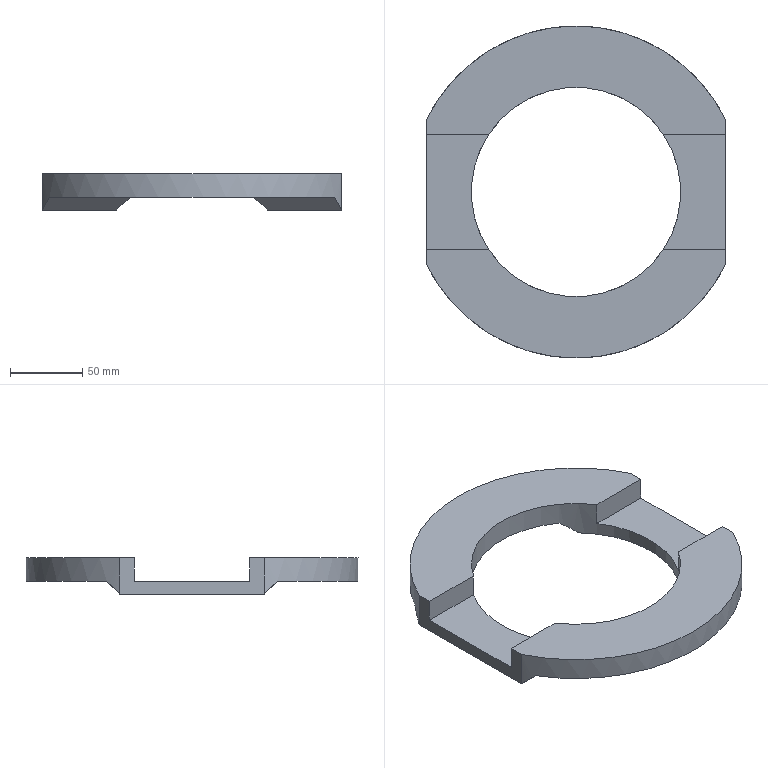Part | NX | features 掩护梁 2 | 1 solid | 21 faces | box 207.123 x 230 x 25 mm | volume 362169 mm3 | plane 18 | cylinder 3 | commonest cylinder face diameters 230 x2 145 x1
STEP:
#1=CARTESIAN_POINT('',(-1870.619,3715.447,-663.771));
#2=VERTEX_POINT('',#1);
#3=CARTESIAN_POINT('',(-1870.619,3715.447,-688.771));
#4=VERTEX_POINT('',#3);
#5=CARTESIAN_POINT('',(-1870.619,3715.447,-688.771));
#6=DIRECTION('',(0.,0.,1.));
#7=VECTOR('',#6,1000.);
#8=LINE('',#5,#7);
#9=EDGE_CURVE('',#2,#4,#8,.F.);
#10=ORIENTED_EDGE('',*,*,#9,.F.);
#11=CARTESIAN_POINT('',(-2077.742,3715.447,-663.771));
#12=VERTEX_POINT('',#11);
#13=CARTESIAN_POINT('',(-1974.181,3765.447,-663.771));
#14=DIRECTION('',(0.,0.,1.));
#15=DIRECTION('',(1.,0.,0.));
#16=AXIS2_PLACEMENT_3D('',#13,#14,#15);
#17=CIRCLE('',#16,115.);
#18=EDGE_CURVE('',#12,#2,#17,.T.);
#19=ORIENTED_EDGE('',*,*,#18,.F.);
#20=CARTESIAN_POINT('',(-2077.742,3715.447,-688.771));
#21=VERTEX_POINT('',#20);
#22=CARTESIAN_POINT('',(-2077.742,3715.447,-688.771));
#23=DIRECTION('',(0.,0.,1.));
#24=VECTOR('',#23,1000.);
#25=LINE('',#22,#24);
#26=EDGE_CURVE('',#21,#12,#25,.T.);
#27=ORIENTED_EDGE('',*,*,#26,.F.);
#28=CARTESIAN_POINT('',(-2072.893,3706.447,-679.771));
#29=VERTEX_POINT('',#28);
#30=CARTESIAN_POINT('',(-1974.181,3765.447,-738.771));
#31=DIRECTION('',(0.,-0.7071,-0.7071));
#32=DIRECTION('',(0.,-0.7071,0.7071));
#33=AXIS2_PLACEMENT_3D('',#30,#31,#32);
#34=ELLIPSE('',#33,162.635,115.);
#35=EDGE_CURVE('',#21,#29,#34,.F.);
#36=ORIENTED_EDGE('',*,*,#35,.T.);
#37=CARTESIAN_POINT('',(-1875.469,3706.447,-679.771));
#38=VERTEX_POINT('',#37);
#39=CARTESIAN_POINT('',(-1974.181,3765.447,-679.771));
#40=DIRECTION('',(0.,0.,-1.));
#41=DIRECTION('',(-1.,0.,0.));
#42=AXIS2_PLACEMENT_3D('',#39,#40,#41);
#43=CIRCLE('',#42,115.);
#44=EDGE_CURVE('',#29,#38,#43,.F.);
#45=ORIENTED_EDGE('',*,*,#44,.T.);
#46=CARTESIAN_POINT('',(-1974.181,3765.447,-738.771));
#47=DIRECTION('',(0.,-0.7071,-0.7071));
#48=DIRECTION('',(0.,-0.7071,0.7071));
#49=AXIS2_PLACEMENT_3D('',#46,#47,#48);
#50=ELLIPSE('',#49,162.635,115.);
#51=EDGE_CURVE('',#38,#4,#50,.F.);
#52=ORIENTED_EDGE('',*,*,#51,.T.);
#53=EDGE_LOOP('',(#10,#19,#27,#36,#45,#52));
#54=FACE_BOUND('',#53,.T.);
#55=CARTESIAN_POINT('',(-1974.181,3765.447,-688.771));
#56=DIRECTION('',(0.,0.,1.));
#57=DIRECTION('',(1.,0.,0.));
#58=AXIS2_PLACEMENT_3D('',#55,#56,#57);
#59=CYLINDRICAL_SURFACE('',#58,115.);
#60=ADVANCED_FACE('',(#54),#59,.T.);
#61=CARTESIAN_POINT('',(-1870.619,3815.447,-688.771));
#62=VERTEX_POINT('',#61);
#63=CARTESIAN_POINT('',(-1870.619,3815.447,-663.771));
#64=VERTEX_POINT('',#63);
#65=CARTESIAN_POINT('',(-1870.619,3815.447,-688.771));
#66=DIRECTION('',(0.,0.,1.));
#67=VECTOR('',#66,1000.);
#68=LINE('',#65,#67);
#69=EDGE_CURVE('',#62,#64,#68,.T.);
#70=ORIENTED_EDGE('',*,*,#69,.F.);
#71=CARTESIAN_POINT('',(-1875.469,3824.447,-679.771));
#72=VERTEX_POINT('',#71);
#73=CARTESIAN_POINT('',(-1974.181,3765.447,-738.771));
#74=DIRECTION('',(0.,0.7071,-0.7071));
#75=DIRECTION('',(0.,0.7071,0.7071));
#76=AXIS2_PLACEMENT_3D('',#73,#74,#75);
#77=ELLIPSE('',#76,162.635,115.);
#78=EDGE_CURVE('',#62,#72,#77,.F.);
#79=ORIENTED_EDGE('',*,*,#78,.T.);
#80=CARTESIAN_POINT('',(-2072.893,3824.447,-679.771));
#81=VERTEX_POINT('',#80);
#82=CARTESIAN_POINT('',(-1974.181,3765.447,-679.771));
#83=DIRECTION('',(0.,0.,-1.));
#84=DIRECTION('',(-1.,0.,0.));
#85=AXIS2_PLACEMENT_3D('',#82,#83,#84);
#86=CIRCLE('',#85,115.);
#87=EDGE_CURVE('',#72,#81,#86,.F.);
#88=ORIENTED_EDGE('',*,*,#87,.T.);
#89=CARTESIAN_POINT('',(-2077.742,3815.447,-688.771));
#90=VERTEX_POINT('',#89);
#91=CARTESIAN_POINT('',(-1974.181,3765.447,-738.771));
#92=DIRECTION('',(0.,0.7071,-0.7071));
#93=DIRECTION('',(0.,0.7071,0.7071));
#94=AXIS2_PLACEMENT_3D('',#91,#92,#93);
#95=ELLIPSE('',#94,162.635,115.);
#96=EDGE_CURVE('',#81,#90,#95,.F.);
#97=ORIENTED_EDGE('',*,*,#96,.T.);
#98=CARTESIAN_POINT('',(-2077.742,3815.447,-663.771));
#99=VERTEX_POINT('',#98);
#100=CARTESIAN_POINT('',(-2077.742,3815.447,-688.771));
#101=DIRECTION('',(0.,0.,1.));
#102=VECTOR('',#101,1000.);
#103=LINE('',#100,#102);
#104=EDGE_CURVE('',#99,#90,#103,.F.);
#105=ORIENTED_EDGE('',*,*,#104,.F.);
#106=CARTESIAN_POINT('',(-1974.181,3765.447,-663.771));
#107=DIRECTION('',(0.,0.,1.));
#108=DIRECTION('',(1.,0.,0.));
#109=AXIS2_PLACEMENT_3D('',#106,#107,#108);
#110=CIRCLE('',#109,115.);
#111=EDGE_CURVE('',#64,#99,#110,.T.);
#112=ORIENTED_EDGE('',*,*,#111,.F.);
#113=EDGE_LOOP('',(#70,#79,#88,#97,#105,#112));
#114=FACE_BOUND('',#113,.T.);
#115=CARTESIAN_POINT('',(-1974.181,3765.447,-688.771));
#116=DIRECTION('',(0.,0.,1.));
#117=DIRECTION('',(1.,0.,0.));
#118=AXIS2_PLACEMENT_3D('',#115,#116,#117);
#119=CYLINDRICAL_SURFACE('',#118,115.);
#120=ADVANCED_FACE('',(#114),#119,.T.);
#121=CARTESIAN_POINT('',(-2026.681,3715.447,-688.771));
#122=VERTEX_POINT('',#121);
#123=CARTESIAN_POINT('',(-2140.181,3715.447,-688.771));
#124=DIRECTION('',(1.,0.,0.));
#125=VECTOR('',#124,1000.);
#126=LINE('',#123,#125);
#127=EDGE_CURVE('',#21,#122,#126,.T.);
#128=ORIENTED_EDGE('',*,*,#127,.F.);
#129=CARTESIAN_POINT('',(-2077.742,3884.447,-688.771));
#130=DIRECTION('',(0.,-1.,0.));
#131=VECTOR('',#130,1000.);
#132=LINE('',#129,#131);
#133=EDGE_CURVE('',#90,#21,#132,.T.);
#134=ORIENTED_EDGE('',*,*,#133,.F.);
#135=CARTESIAN_POINT('',(-2026.681,3815.447,-688.771));
#136=VERTEX_POINT('',#135);
#137=CARTESIAN_POINT('',(-2140.181,3815.447,-688.771));
#138=DIRECTION('',(1.,0.,0.));
#139=VECTOR('',#138,1000.);
#140=LINE('',#137,#139);
#141=EDGE_CURVE('',#90,#136,#140,.T.);
#142=ORIENTED_EDGE('',*,*,#141,.T.);
#143=CARTESIAN_POINT('',(-1974.181,3765.447,-688.771));
#144=DIRECTION('',(0.,0.,1.));
#145=DIRECTION('',(1.,0.,0.));
#146=AXIS2_PLACEMENT_3D('',#143,#144,#145);
#147=CIRCLE('',#146,72.5);
#148=EDGE_CURVE('',#136,#122,#147,.T.);
#149=ORIENTED_EDGE('',*,*,#148,.T.);
#150=EDGE_LOOP('',(#128,#134,#142,#149));
#151=FACE_BOUND('',#150,.T.);
#152=CARTESIAN_POINT('',(-1974.181,3765.447,-688.771));
#153=DIRECTION('',(0.,0.,1.));
#154=DIRECTION('',(1.,0.,0.));
#155=AXIS2_PLACEMENT_3D('',#152,#153,#154);
#156=PLANE('',#155);
#157=ADVANCED_FACE('',(#151),#156,.F.);
#158=CARTESIAN_POINT('',(-1921.681,3815.447,-688.771));
#159=VERTEX_POINT('',#158);
#160=CARTESIAN_POINT('',(-2140.181,3815.447,-688.771));
#161=DIRECTION('',(1.,0.,0.));
#162=VECTOR('',#161,1000.);
#163=LINE('',#160,#162);
#164=EDGE_CURVE('',#159,#62,#163,.T.);
#165=ORIENTED_EDGE('',*,*,#164,.T.);
#166=CARTESIAN_POINT('',(-1870.619,3884.447,-688.771));
#167=DIRECTION('',(0.,-1.,0.));
#168=VECTOR('',#167,1000.);
#169=LINE('',#166,#168);
#170=EDGE_CURVE('',#62,#4,#169,.T.);
#171=ORIENTED_EDGE('',*,*,#170,.T.);
#172=CARTESIAN_POINT('',(-1921.681,3715.447,-688.771));
#173=VERTEX_POINT('',#172);
#174=CARTESIAN_POINT('',(-2140.181,3715.447,-688.771));
#175=DIRECTION('',(1.,0.,0.));
#176=VECTOR('',#175,1000.);
#177=LINE('',#174,#176);
#178=EDGE_CURVE('',#173,#4,#177,.T.);
#179=ORIENTED_EDGE('',*,*,#178,.F.);
#180=CARTESIAN_POINT('',(-1974.181,3765.447,-688.771));
#181=DIRECTION('',(0.,0.,1.));
#182=DIRECTION('',(1.,0.,0.));
#183=AXIS2_PLACEMENT_3D('',#180,#181,#182);
#184=CIRCLE('',#183,72.5);
#185=EDGE_CURVE('',#173,#159,#184,.T.);
#186=ORIENTED_EDGE('',*,*,#185,.T.);
#187=EDGE_LOOP('',(#165,#171,#179,#186));
#188=FACE_BOUND('',#187,.T.);
#189=CARTESIAN_POINT('',(-1974.181,3765.447,-688.771));
#190=DIRECTION('',(0.,0.,1.));
#191=DIRECTION('',(1.,0.,0.));
#192=AXIS2_PLACEMENT_3D('',#189,#190,#191);
#193=PLANE('',#192);
#194=ADVANCED_FACE('',(#188),#193,.F.);
#195=CARTESIAN_POINT('',(-1870.619,3725.447,-663.771));
#196=VERTEX_POINT('',#195);
#197=CARTESIAN_POINT('',(-1870.619,3884.447,-663.771));
#198=DIRECTION('',(0.,-1.,0.));
#199=VECTOR('',#198,1000.);
#200=LINE('',#197,#199);
#201=EDGE_CURVE('',#196,#2,#200,.T.);
#202=ORIENTED_EDGE('',*,*,#201,.F.);
#203=CARTESIAN_POINT('',(-1913.714,3725.447,-663.771));
#204=VERTEX_POINT('',#203);
#205=CARTESIAN_POINT('',(-2140.181,3725.447,-663.771));
#206=DIRECTION('',(1.,0.,0.));
#207=VECTOR('',#206,1000.);
#208=LINE('',#205,#207);
#209=EDGE_CURVE('',#204,#196,#208,.T.);
#210=ORIENTED_EDGE('',*,*,#209,.F.);
#211=CARTESIAN_POINT('',(-2034.648,3725.447,-663.771));
#212=VERTEX_POINT('',#211);
#213=CARTESIAN_POINT('',(-1974.181,3765.447,-663.771));
#214=DIRECTION('',(0.,0.,1.));
#215=DIRECTION('',(1.,0.,0.));
#216=AXIS2_PLACEMENT_3D('',#213,#214,#215);
#217=CIRCLE('',#216,72.5);
#218=EDGE_CURVE('',#212,#204,#217,.T.);
#219=ORIENTED_EDGE('',*,*,#218,.F.);
#220=CARTESIAN_POINT('',(-2077.742,3725.447,-663.771));
#221=VERTEX_POINT('',#220);
#222=CARTESIAN_POINT('',(-2140.181,3725.447,-663.771));
#223=DIRECTION('',(1.,0.,0.));
#224=VECTOR('',#223,1000.);
#225=LINE('',#222,#224);
#226=EDGE_CURVE('',#221,#212,#225,.T.);
#227=ORIENTED_EDGE('',*,*,#226,.F.);
#228=CARTESIAN_POINT('',(-2077.742,3884.447,-663.771));
#229=DIRECTION('',(0.,-1.,0.));
#230=VECTOR('',#229,1000.);
#231=LINE('',#228,#230);
#232=EDGE_CURVE('',#221,#12,#231,.T.);
#233=ORIENTED_EDGE('',*,*,#232,.T.);
#234=ORIENTED_EDGE('',*,*,#18,.T.);
#235=EDGE_LOOP('',(#202,#210,#219,#227,#233,#234));
#236=FACE_BOUND('',#235,.T.);
#237=CARTESIAN_POINT('',(-1974.181,3765.447,-663.771));
#238=DIRECTION('',(0.,0.,1.));
#239=DIRECTION('',(1.,0.,0.));
#240=AXIS2_PLACEMENT_3D('',#237,#238,#239);
#241=PLANE('',#240);
#242=ADVANCED_FACE('',(#236),#241,.T.);
#243=CARTESIAN_POINT('',(-1870.619,3805.447,-663.771));
#244=VERTEX_POINT('',#243);
#245=CARTESIAN_POINT('',(-1870.619,3884.447,-663.771));
#246=DIRECTION('',(0.,-1.,0.));
#247=VECTOR('',#246,1000.);
#248=LINE('',#245,#247);
#249=EDGE_CURVE('',#64,#244,#248,.T.);
#250=ORIENTED_EDGE('',*,*,#249,.F.);
#251=ORIENTED_EDGE('',*,*,#111,.T.);
#252=CARTESIAN_POINT('',(-2077.742,3805.447,-663.771));
#253=VERTEX_POINT('',#252);
#254=CARTESIAN_POINT('',(-2077.742,3884.447,-663.771));
#255=DIRECTION('',(0.,-1.,0.));
#256=VECTOR('',#255,1000.);
#257=LINE('',#254,#256);
#258=EDGE_CURVE('',#99,#253,#257,.T.);
#259=ORIENTED_EDGE('',*,*,#258,.T.);
#260=CARTESIAN_POINT('',(-2034.648,3805.447,-663.771));
#261=VERTEX_POINT('',#260);
#262=CARTESIAN_POINT('',(-2140.181,3805.447,-663.771));
#263=DIRECTION('',(1.,0.,0.));
#264=VECTOR('',#263,1000.);
#265=LINE('',#262,#264);
#266=EDGE_CURVE('',#253,#261,#265,.T.);
#267=ORIENTED_EDGE('',*,*,#266,.T.);
#268=CARTESIAN_POINT('',(-1913.714,3805.447,-663.771));
#269=VERTEX_POINT('',#268);
#270=CARTESIAN_POINT('',(-1974.181,3765.447,-663.771));
#271=DIRECTION('',(0.,0.,1.));
#272=DIRECTION('',(1.,0.,0.));
#273=AXIS2_PLACEMENT_3D('',#270,#271,#272);
#274=CIRCLE('',#273,72.5);
#275=EDGE_CURVE('',#269,#261,#274,.T.);
#276=ORIENTED_EDGE('',*,*,#275,.F.);
#277=CARTESIAN_POINT('',(-2140.181,3805.447,-663.771));
#278=DIRECTION('',(1.,0.,0.));
#279=VECTOR('',#278,1000.);
#280=LINE('',#277,#279);
#281=EDGE_CURVE('',#269,#244,#280,.T.);
#282=ORIENTED_EDGE('',*,*,#281,.T.);
#283=EDGE_LOOP('',(#250,#251,#259,#267,#276,#282));
#284=FACE_BOUND('',#283,.T.);
#285=CARTESIAN_POINT('',(-1974.181,3765.447,-663.771));
#286=DIRECTION('',(0.,0.,1.));
#287=DIRECTION('',(1.,0.,0.));
#288=AXIS2_PLACEMENT_3D('',#285,#286,#287);
#289=PLANE('',#288);
#290=ADVANCED_FACE('',(#284),#289,.T.);
#291=CARTESIAN_POINT('',(-1932.047,3706.447,-679.771));
#292=VERTEX_POINT('',#291);
#293=CARTESIAN_POINT('',(-1974.181,3765.447,-738.771));
#294=DIRECTION('',(0.,-0.7071,-0.7071));
#295=DIRECTION('',(0.,-0.7071,0.7071));
#296=AXIS2_PLACEMENT_3D('',#293,#294,#295);
#297=ELLIPSE('',#296,102.53,72.5);
#298=EDGE_CURVE('',#292,#173,#297,.F.);
#299=ORIENTED_EDGE('',*,*,#298,.F.);
#300=CARTESIAN_POINT('',(-2016.315,3706.447,-679.771));
#301=VERTEX_POINT('',#300);
#302=CARTESIAN_POINT('',(-1974.181,3765.447,-679.771));
#303=DIRECTION('',(0.,0.,-1.));
#304=DIRECTION('',(-1.,0.,0.));
#305=AXIS2_PLACEMENT_3D('',#302,#303,#304);
#306=CIRCLE('',#305,72.5);
#307=EDGE_CURVE('',#301,#292,#306,.F.);
#308=ORIENTED_EDGE('',*,*,#307,.F.);
#309=CARTESIAN_POINT('',(-1974.181,3765.447,-738.771));
#310=DIRECTION('',(0.,-0.7071,-0.7071));
#311=DIRECTION('',(0.,-0.7071,0.7071));
#312=AXIS2_PLACEMENT_3D('',#309,#310,#311);
#313=ELLIPSE('',#312,102.53,72.5);
#314=EDGE_CURVE('',#122,#301,#313,.F.);
#315=ORIENTED_EDGE('',*,*,#314,.F.);
#316=ORIENTED_EDGE('',*,*,#148,.F.);
#317=CARTESIAN_POINT('',(-2016.315,3824.447,-679.771));
#318=VERTEX_POINT('',#317);
#319=CARTESIAN_POINT('',(-1974.181,3765.447,-738.771));
#320=DIRECTION('',(0.,0.7071,-0.7071));
#321=DIRECTION('',(0.,0.7071,0.7071));
#322=AXIS2_PLACEMENT_3D('',#319,#320,#321);
#323=ELLIPSE('',#322,102.53,72.5);
#324=EDGE_CURVE('',#318,#136,#323,.F.);
#325=ORIENTED_EDGE('',*,*,#324,.F.);
#326=CARTESIAN_POINT('',(-1932.047,3824.447,-679.771));
#327=VERTEX_POINT('',#326);
#328=CARTESIAN_POINT('',(-1974.181,3765.447,-679.771));
#329=DIRECTION('',(0.,0.,-1.));
#330=DIRECTION('',(-1.,0.,0.));
#331=AXIS2_PLACEMENT_3D('',#328,#329,#330);
#332=CIRCLE('',#331,72.5);
#333=EDGE_CURVE('',#327,#318,#332,.F.);
#334=ORIENTED_EDGE('',*,*,#333,.F.);
#335=CARTESIAN_POINT('',(-1974.181,3765.447,-738.771));
#336=DIRECTION('',(0.,0.7071,-0.7071));
#337=DIRECTION('',(0.,0.7071,0.7071));
#338=AXIS2_PLACEMENT_3D('',#335,#336,#337);
#339=ELLIPSE('',#338,102.53,72.5);
#340=EDGE_CURVE('',#159,#327,#339,.F.);
#341=ORIENTED_EDGE('',*,*,#340,.F.);
#342=ORIENTED_EDGE('',*,*,#185,.F.);
#343=EDGE_LOOP('',(#299,#308,#315,#316,#325,#334,#341,#342));
#344=FACE_BOUND('',#343,.T.);
#345=CARTESIAN_POINT('',(-2034.648,3725.447,-679.771));
#346=VERTEX_POINT('',#345);
#347=CARTESIAN_POINT('',(-2034.648,3725.447,-688.771));
#348=DIRECTION('',(0.,0.,1.));
#349=VECTOR('',#348,1000.);
#350=LINE('',#347,#349);
#351=EDGE_CURVE('',#212,#346,#350,.F.);
#352=ORIENTED_EDGE('',*,*,#351,.F.);
#353=ORIENTED_EDGE('',*,*,#218,.T.);
#354=CARTESIAN_POINT('',(-1913.714,3725.447,-679.771));
#355=VERTEX_POINT('',#354);
#356=CARTESIAN_POINT('',(-1913.714,3725.447,-688.771));
#357=DIRECTION('',(0.,0.,1.));
#358=VECTOR('',#357,1000.);
#359=LINE('',#356,#358);
#360=EDGE_CURVE('',#355,#204,#359,.T.);
#361=ORIENTED_EDGE('',*,*,#360,.F.);
#362=CARTESIAN_POINT('',(-1913.714,3805.447,-679.771));
#363=VERTEX_POINT('',#362);
#364=CARTESIAN_POINT('',(-1974.181,3765.447,-679.771));
#365=DIRECTION('',(0.,0.,1.));
#366=DIRECTION('',(1.,0.,0.));
#367=AXIS2_PLACEMENT_3D('',#364,#365,#366);
#368=CIRCLE('',#367,72.5);
#369=EDGE_CURVE('',#363,#355,#368,.F.);
#370=ORIENTED_EDGE('',*,*,#369,.F.);
#371=CARTESIAN_POINT('',(-1913.714,3805.447,-688.771));
#372=DIRECTION('',(0.,0.,1.));
#373=VECTOR('',#372,1000.);
#374=LINE('',#371,#373);
#375=EDGE_CURVE('',#269,#363,#374,.F.);
#376=ORIENTED_EDGE('',*,*,#375,.F.);
#377=ORIENTED_EDGE('',*,*,#275,.T.);
#378=CARTESIAN_POINT('',(-2034.648,3805.447,-679.771));
#379=VERTEX_POINT('',#378);
#380=CARTESIAN_POINT('',(-2034.648,3805.447,-688.771));
#381=DIRECTION('',(0.,0.,1.));
#382=VECTOR('',#381,1000.);
#383=LINE('',#380,#382);
#384=EDGE_CURVE('',#379,#261,#383,.T.);
#385=ORIENTED_EDGE('',*,*,#384,.F.);
#386=CARTESIAN_POINT('',(-1974.181,3765.447,-679.771));
#387=DIRECTION('',(0.,0.,1.));
#388=DIRECTION('',(1.,0.,0.));
#389=AXIS2_PLACEMENT_3D('',#386,#387,#388);
#390=CIRCLE('',#389,72.5);
#391=EDGE_CURVE('',#346,#379,#390,.F.);
#392=ORIENTED_EDGE('',*,*,#391,.F.);
#393=EDGE_LOOP('',(#352,#353,#361,#370,#376,#377,#385,#392));
#394=FACE_BOUND('',#393,.T.);
#395=CARTESIAN_POINT('',(-1974.181,3765.447,-688.771));
#396=DIRECTION('',(0.,0.,1.));
#397=DIRECTION('',(1.,0.,0.));
#398=AXIS2_PLACEMENT_3D('',#395,#396,#397);
#399=CYLINDRICAL_SURFACE('',#398,72.5);
#400=ADVANCED_FACE('',(#344,#394),#399,.F.);
#401=CARTESIAN_POINT('',(-2140.181,3824.447,-679.771));
#402=DIRECTION('',(1.,0.,0.));
#403=VECTOR('',#402,1000.);
#404=LINE('',#401,#403);
#405=EDGE_CURVE('',#81,#318,#404,.T.);
#406=ORIENTED_EDGE('',*,*,#405,.T.);
#407=ORIENTED_EDGE('',*,*,#324,.T.);
#408=ORIENTED_EDGE('',*,*,#141,.F.);
#409=ORIENTED_EDGE('',*,*,#96,.F.);
#410=EDGE_LOOP('',(#406,#407,#408,#409));
#411=FACE_BOUND('',#410,.T.);
#412=CARTESIAN_POINT('',(-2140.181,3815.447,-688.771));
#413=DIRECTION('',(0.,0.7071,-0.7071));
#414=DIRECTION('',(0.,0.7071,0.7071));
#415=AXIS2_PLACEMENT_3D('',#412,#413,#414);
#416=PLANE('',#415);
#417=ADVANCED_FACE('',(#411),#416,.T.);
#418=ORIENTED_EDGE('',*,*,#164,.F.);
#419=ORIENTED_EDGE('',*,*,#340,.T.);
#420=CARTESIAN_POINT('',(-2140.181,3824.447,-679.771));
#421=DIRECTION('',(1.,0.,0.));
#422=VECTOR('',#421,1000.);
#423=LINE('',#420,#422);
#424=EDGE_CURVE('',#327,#72,#423,.T.);
#425=ORIENTED_EDGE('',*,*,#424,.T.);
#426=ORIENTED_EDGE('',*,*,#78,.F.);
#427=EDGE_LOOP('',(#418,#419,#425,#426));
#428=FACE_BOUND('',#427,.T.);
#429=CARTESIAN_POINT('',(-2140.181,3815.447,-688.771));
#430=DIRECTION('',(0.,0.7071,-0.7071));
#431=DIRECTION('',(0.,0.7071,0.7071));
#432=AXIS2_PLACEMENT_3D('',#429,#430,#431);
#433=PLANE('',#432);
#434=ADVANCED_FACE('',(#428),#433,.T.);
#435=ORIENTED_EDGE('',*,*,#424,.F.);
#436=ORIENTED_EDGE('',*,*,#333,.T.);
#437=ORIENTED_EDGE('',*,*,#405,.F.);
#438=ORIENTED_EDGE('',*,*,#87,.F.);
#439=EDGE_LOOP('',(#435,#436,#437,#438));
#440=FACE_BOUND('',#439,.T.);
#441=CARTESIAN_POINT('',(-2140.181,3824.447,-679.771));
#442=DIRECTION('',(0.,0.,-1.));
#443=DIRECTION('',(-1.,0.,0.));
#444=AXIS2_PLACEMENT_3D('',#441,#442,#443);
#445=PLANE('',#444);
#446=ADVANCED_FACE('',(#440),#445,.T.);
#447=CARTESIAN_POINT('',(-2140.181,3706.447,-679.771));
#448=DIRECTION('',(1.,0.,0.));
#449=VECTOR('',#448,1000.);
#450=LINE('',#447,#449);
#451=EDGE_CURVE('',#29,#301,#450,.T.);
#452=ORIENTED_EDGE('',*,*,#451,.T.);
#453=ORIENTED_EDGE('',*,*,#307,.T.);
#454=CARTESIAN_POINT('',(-2140.181,3706.447,-679.771));
#455=DIRECTION('',(1.,0.,0.));
#456=VECTOR('',#455,1000.);
#457=LINE('',#454,#456);
#458=EDGE_CURVE('',#292,#38,#457,.T.);
#459=ORIENTED_EDGE('',*,*,#458,.T.);
#460=ORIENTED_EDGE('',*,*,#44,.F.);
#461=EDGE_LOOP('',(#452,#453,#459,#460));
#462=FACE_BOUND('',#461,.T.);
#463=CARTESIAN_POINT('',(-2140.181,3706.447,-679.771));
#464=DIRECTION('',(0.,0.,-1.));
#465=DIRECTION('',(-1.,0.,0.));
#466=AXIS2_PLACEMENT_3D('',#463,#464,#465);
#467=PLANE('',#466);
#468=ADVANCED_FACE('',(#462),#467,.T.);
#469=ORIENTED_EDGE('',*,*,#458,.F.);
#470=ORIENTED_EDGE('',*,*,#298,.T.);
#471=ORIENTED_EDGE('',*,*,#178,.T.);
#472=ORIENTED_EDGE('',*,*,#51,.F.);
#473=EDGE_LOOP('',(#469,#470,#471,#472));
#474=FACE_BOUND('',#473,.T.);
#475=CARTESIAN_POINT('',(-2140.181,3715.447,-688.771));
#476=DIRECTION('',(0.,-0.7071,-0.7071));
#477=DIRECTION('',(0.,0.7071,-0.7071));
#478=AXIS2_PLACEMENT_3D('',#475,#476,#477);
#479=PLANE('',#478);
#480=ADVANCED_FACE('',(#474),#479,.T.);
#481=ORIENTED_EDGE('',*,*,#127,.T.);
#482=ORIENTED_EDGE('',*,*,#314,.T.);
#483=ORIENTED_EDGE('',*,*,#451,.F.);
#484=ORIENTED_EDGE('',*,*,#35,.F.);
#485=EDGE_LOOP('',(#481,#482,#483,#484));
#486=FACE_BOUND('',#485,.T.);
#487=CARTESIAN_POINT('',(-2140.181,3715.447,-688.771));
#488=DIRECTION('',(0.,-0.7071,-0.7071));
#489=DIRECTION('',(0.,0.7071,-0.7071));
#490=AXIS2_PLACEMENT_3D('',#487,#488,#489);
#491=PLANE('',#490);
#492=ADVANCED_FACE('',(#486),#491,.T.);
#493=CARTESIAN_POINT('',(-1870.619,3805.447,-679.771));
#494=VERTEX_POINT('',#493);
#495=CARTESIAN_POINT('',(-1870.619,3725.447,-679.771));
#496=VERTEX_POINT('',#495);
#497=CARTESIAN_POINT('',(-1870.619,3805.447,-679.771));
#498=DIRECTION('',(0.,-1.,0.));
#499=VECTOR('',#498,1000.);
#500=LINE('',#497,#499);
#501=EDGE_CURVE('',#494,#496,#500,.T.);
#502=ORIENTED_EDGE('',*,*,#501,.F.);
#503=CARTESIAN_POINT('',(-2140.181,3805.447,-679.771));
#504=DIRECTION('',(1.,0.,0.));
#505=VECTOR('',#504,1000.);
#506=LINE('',#503,#505);
#507=EDGE_CURVE('',#363,#494,#506,.T.);
#508=ORIENTED_EDGE('',*,*,#507,.F.);
#509=ORIENTED_EDGE('',*,*,#369,.T.);
#510=CARTESIAN_POINT('',(-2140.181,3725.447,-679.771));
#511=DIRECTION('',(1.,0.,0.));
#512=VECTOR('',#511,1000.);
#513=LINE('',#510,#512);
#514=EDGE_CURVE('',#355,#496,#513,.T.);
#515=ORIENTED_EDGE('',*,*,#514,.T.);
#516=EDGE_LOOP('',(#502,#508,#509,#515));
#517=FACE_BOUND('',#516,.T.);
#518=CARTESIAN_POINT('',(-2140.181,3805.447,-679.771));
#519=DIRECTION('',(0.,0.,1.));
#520=DIRECTION('',(1.,0.,0.));
#521=AXIS2_PLACEMENT_3D('',#518,#519,#520);
#522=PLANE('',#521);
#523=ADVANCED_FACE('',(#517),#522,.T.);
#524=CARTESIAN_POINT('',(-1870.619,3805.447,-679.771));
#525=DIRECTION('',(0.,0.,-1.));
#526=VECTOR('',#525,1000.);
#527=LINE('',#524,#526);
#528=EDGE_CURVE('',#244,#494,#527,.T.);
#529=ORIENTED_EDGE('',*,*,#528,.F.);
#530=ORIENTED_EDGE('',*,*,#281,.F.);
#531=ORIENTED_EDGE('',*,*,#375,.T.);
#532=ORIENTED_EDGE('',*,*,#507,.T.);
#533=EDGE_LOOP('',(#529,#530,#531,#532));
#534=FACE_BOUND('',#533,.T.);
#535=CARTESIAN_POINT('',(-2140.181,3805.447,-679.771));
#536=DIRECTION('',(0.,-1.,0.));
#537=DIRECTION('',(0.,0.,-1.));
#538=AXIS2_PLACEMENT_3D('',#535,#536,#537);
#539=PLANE('',#538);
#540=ADVANCED_FACE('',(#534),#539,.T.);
#541=CARTESIAN_POINT('',(-1870.619,3725.447,-679.771));
#542=DIRECTION('',(0.,0.,1.));
#543=VECTOR('',#542,1000.);
#544=LINE('',#541,#543);
#545=EDGE_CURVE('',#496,#196,#544,.T.);
#546=ORIENTED_EDGE('',*,*,#545,.F.);
#547=ORIENTED_EDGE('',*,*,#514,.F.);
#548=ORIENTED_EDGE('',*,*,#360,.T.);
#549=ORIENTED_EDGE('',*,*,#209,.T.);
#550=EDGE_LOOP('',(#546,#547,#548,#549));
#551=FACE_BOUND('',#550,.T.);
#552=CARTESIAN_POINT('',(-2140.181,3725.447,-679.771));
#553=DIRECTION('',(0.,1.,0.));
#554=DIRECTION('',(0.,0.,1.));
#555=AXIS2_PLACEMENT_3D('',#552,#553,#554);
#556=PLANE('',#555);
#557=ADVANCED_FACE('',(#551),#556,.T.);
#558=CARTESIAN_POINT('',(-2077.742,3725.447,-679.771));
#559=VERTEX_POINT('',#558);
#560=CARTESIAN_POINT('',(-2077.742,3725.447,-679.771));
#561=DIRECTION('',(0.,0.,-1.));
#562=VECTOR('',#561,1000.);
#563=LINE('',#560,#562);
#564=EDGE_CURVE('',#221,#559,#563,.T.);
#565=ORIENTED_EDGE('',*,*,#564,.F.);
#566=ORIENTED_EDGE('',*,*,#226,.T.);
#567=ORIENTED_EDGE('',*,*,#351,.T.);
#568=CARTESIAN_POINT('',(-2140.181,3725.447,-679.771));
#569=DIRECTION('',(1.,0.,0.));
#570=VECTOR('',#569,1000.);
#571=LINE('',#568,#570);
#572=EDGE_CURVE('',#559,#346,#571,.T.);
#573=ORIENTED_EDGE('',*,*,#572,.F.);
#574=EDGE_LOOP('',(#565,#566,#567,#573));
#575=FACE_BOUND('',#574,.T.);
#576=CARTESIAN_POINT('',(-2140.181,3725.447,-679.771));
#577=DIRECTION('',(0.,1.,0.));
#578=DIRECTION('',(0.,0.,1.));
#579=AXIS2_PLACEMENT_3D('',#576,#577,#578);
#580=PLANE('',#579);
#581=ADVANCED_FACE('',(#575),#580,.T.);
#582=CARTESIAN_POINT('',(-2077.742,3805.447,-679.771));
#583=VERTEX_POINT('',#582);
#584=CARTESIAN_POINT('',(-2077.742,3805.447,-679.771));
#585=DIRECTION('',(0.,0.,1.));
#586=VECTOR('',#585,1000.);
#587=LINE('',#584,#586);
#588=EDGE_CURVE('',#583,#253,#587,.T.);
#589=ORIENTED_EDGE('',*,*,#588,.F.);
#590=CARTESIAN_POINT('',(-2140.181,3805.447,-679.771));
#591=DIRECTION('',(1.,0.,0.));
#592=VECTOR('',#591,1000.);
#593=LINE('',#590,#592);
#594=EDGE_CURVE('',#583,#379,#593,.T.);
#595=ORIENTED_EDGE('',*,*,#594,.T.);
#596=ORIENTED_EDGE('',*,*,#384,.T.);
#597=ORIENTED_EDGE('',*,*,#266,.F.);
#598=EDGE_LOOP('',(#589,#595,#596,#597));
#599=FACE_BOUND('',#598,.T.);
#600=CARTESIAN_POINT('',(-2140.181,3805.447,-679.771));
#601=DIRECTION('',(0.,-1.,0.));
#602=DIRECTION('',(0.,0.,-1.));
#603=AXIS2_PLACEMENT_3D('',#600,#601,#602);
#604=PLANE('',#603);
#605=ADVANCED_FACE('',(#599),#604,.T.);
#606=CARTESIAN_POINT('',(-2077.742,3805.447,-679.771));
#607=DIRECTION('',(0.,1.,0.));
#608=VECTOR('',#607,1000.);
#609=LINE('',#606,#608);
#610=EDGE_CURVE('',#559,#583,#609,.T.);
#611=ORIENTED_EDGE('',*,*,#610,.F.);
#612=ORIENTED_EDGE('',*,*,#572,.T.);
#613=ORIENTED_EDGE('',*,*,#391,.T.);
#614=ORIENTED_EDGE('',*,*,#594,.F.);
#615=EDGE_LOOP('',(#611,#612,#613,#614));
#616=FACE_BOUND('',#615,.T.);
#617=CARTESIAN_POINT('',(-2140.181,3805.447,-679.771));
#618=DIRECTION('',(0.,0.,1.));
#619=DIRECTION('',(1.,0.,0.));
#620=AXIS2_PLACEMENT_3D('',#617,#618,#619);
#621=PLANE('',#620);
#622=ADVANCED_FACE('',(#616),#621,.T.);
#623=ORIENTED_EDGE('',*,*,#104,.T.);
#624=ORIENTED_EDGE('',*,*,#133,.T.);
#625=ORIENTED_EDGE('',*,*,#26,.T.);
#626=ORIENTED_EDGE('',*,*,#232,.F.);
#627=ORIENTED_EDGE('',*,*,#564,.T.);
#628=ORIENTED_EDGE('',*,*,#610,.T.);
#629=ORIENTED_EDGE('',*,*,#588,.T.);
#630=ORIENTED_EDGE('',*,*,#258,.F.);
#631=EDGE_LOOP('',(#623,#624,#625,#626,#627,#628,#629,#630));
#632=FACE_BOUND('',#631,.T.);
#633=CARTESIAN_POINT('',(-2077.742,3884.447,-688.771));
#634=DIRECTION('',(1.,0.,0.));
#635=DIRECTION('',(0.,0.,-1.));
#636=AXIS2_PLACEMENT_3D('',#633,#634,#635);
#637=PLANE('',#636);
#638=ADVANCED_FACE('',(#632),#637,.F.);
#639=ORIENTED_EDGE('',*,*,#9,.T.);
#640=ORIENTED_EDGE('',*,*,#170,.F.);
#641=ORIENTED_EDGE('',*,*,#69,.T.);
#642=ORIENTED_EDGE('',*,*,#249,.T.);
#643=ORIENTED_EDGE('',*,*,#528,.T.);
#644=ORIENTED_EDGE('',*,*,#501,.T.);
#645=ORIENTED_EDGE('',*,*,#545,.T.);
#646=ORIENTED_EDGE('',*,*,#201,.T.);
#647=EDGE_LOOP('',(#639,#640,#641,#642,#643,#644,#645,#646));
#648=FACE_BOUND('',#647,.T.);
#649=CARTESIAN_POINT('',(-1870.619,3884.447,-688.771));
#650=DIRECTION('',(-1.,0.,0.));
#651=DIRECTION('',(0.,0.,1.));
#652=AXIS2_PLACEMENT_3D('',#649,#650,#651);
#653=PLANE('',#652);
#654=ADVANCED_FACE('',(#648),#653,.F.);
#655=CLOSED_SHELL('',(#60,#120,#157,#194,#242,#290,#400,#417,#434,#446,#468,#480,#492,#523,#540,#557,#581,#605,#622,#638,#654));
#656=MANIFOLD_SOLID_BREP('',#655);
#657=(LENGTH_UNIT()NAMED_UNIT(*)SI_UNIT(.MILLI.,.METRE.));
#658=UNCERTAINTY_MEASURE_WITH_UNIT(LENGTH_MEASURE(0.00001),#657,'','');
#659=(NAMED_UNIT(*)PLANE_ANGLE_UNIT()SI_UNIT($,.RADIAN.));
#660=(NAMED_UNIT(*)SI_UNIT($,.STERADIAN.)SOLID_ANGLE_UNIT());
#661=(GEOMETRIC_REPRESENTATION_CONTEXT(3)GLOBAL_UNCERTAINTY_ASSIGNED_CONTEXT((#658))GLOBAL_UNIT_ASSIGNED_CONTEXT((#657,#659,#660))REPRESENTATION_CONTEXT('',''));
#662=ADVANCED_BREP_SHAPE_REPRESENTATION('',(#656),#661);